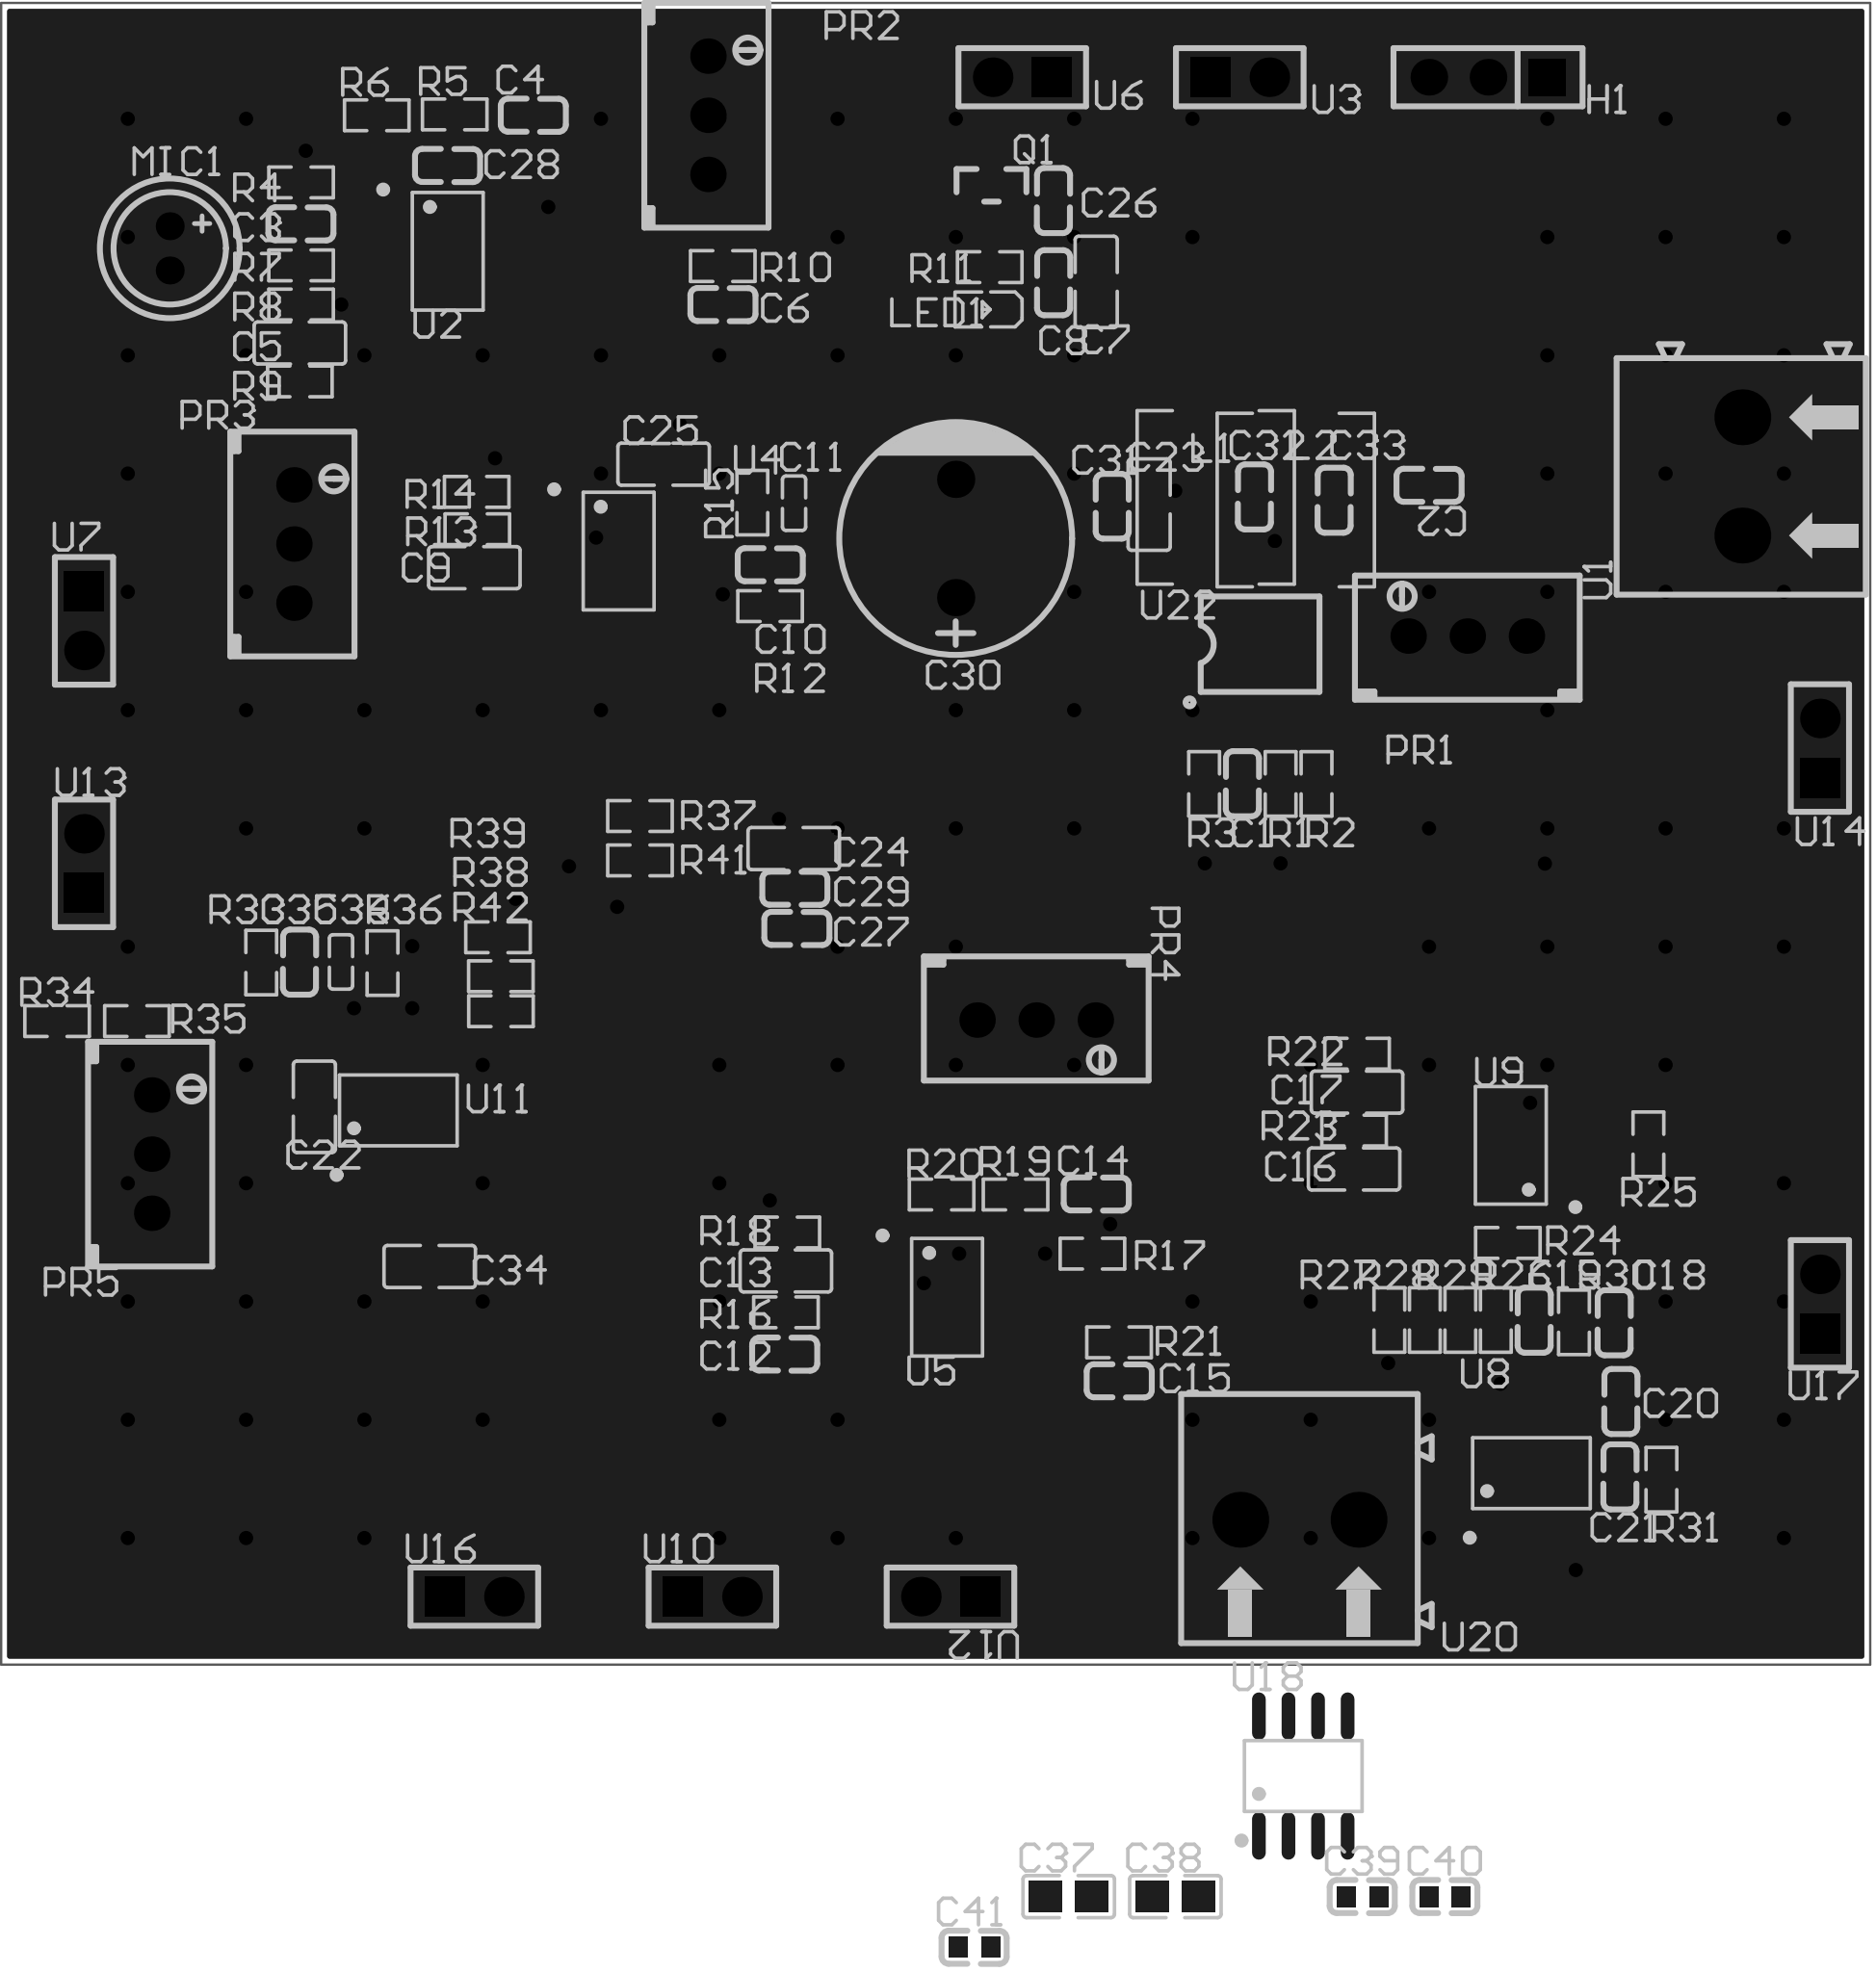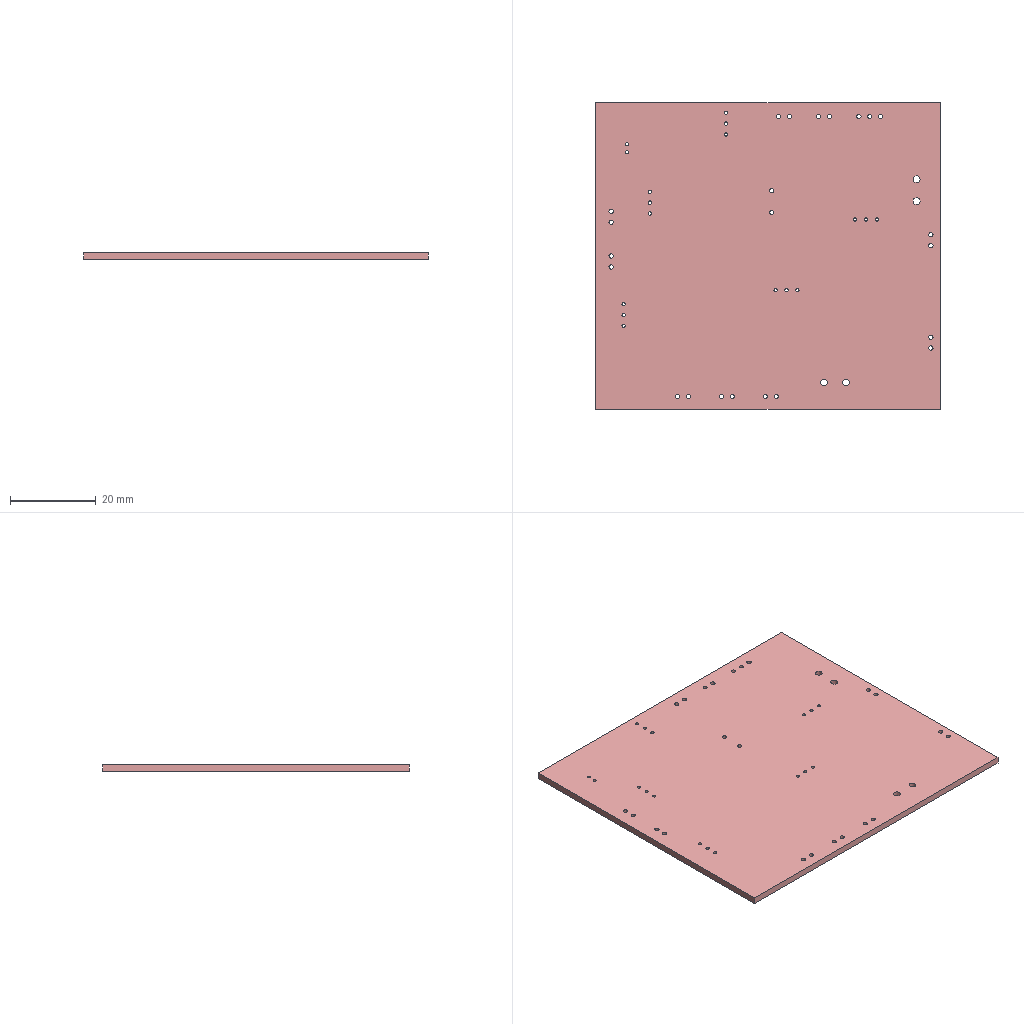Circuit board layout | Altium Designer | box 80.3 x 71.4 x 1.6 mm
Layer stack:
# Altium Designer layer stack of  (unit mm; dielectric type: 0 none, 1 core, 2 prepreg, 3 surface material)
index,name,kind,layer,copper_thickness_mm,dielectric_type,dielectric_thickness_mm,dielectric_material,dielectric_constant
0,Top Paste Mask Layer,other,,,,,,
1,Top Silkscreen Layer,other,,,,,,
2,Top Solder Mask Layer,dielectric,,,3,0.01,,3.3
3,Top Layer,copper,Top Layer,0.035,,,,
4,Dielectric1,dielectric,,,3,1.51,FR4,4.5
5,Bottom Layer,copper,Bottom Layer,0.035,,,,
6,Bottom Solder Mask Layer,dielectric,,,3,0.01,,3.3
7,Bottom Silkscreen Layer,other,,,,,,
8,Bottom Paste Mask Layer,other,,,,,,
# drill layer pairs: low layer,high layer
drill_pair,Top Layer,Bottom Layer
Part placement:
Designator,Comment,Layer,Footprint,Center-X(mm),Center-Y(mm),Rotation
C30,470uF,TopLayer,CAP-TH_BD10.0-P5.00-D1.0-FD,127.987,137.425,90
C31,1uF,TopLayer,C0603,134.709,138.809,90
H1,PM254V-11-03-H85,TopLayer,HDR-TH_3P-P2.54-V-F,150.846,157.237,180
MIC1,GMI6050P-36db,TopLayer,MIC-TH_BD6.0-P1.90-D0.4-L-FD_GMI6050P-2CXXDB,94.234,149.887,270
Q1,AO3401A,TopLayer,SOT-23_L2.9-W1.3-P1.90-LS2.4-BR,129.522,152.595,270
U1,KF128-5.08-2P-AA,TopLayer,CONN-TH_P5.08_KF128-5.08-2P,161.768,140.092,90
U2,NE5532DR,TopLayer,SOIC-8_L4.9-W3.9-P1.27-LS6.0-BL,106.172,149.761,270
U3,ZX-PM2.54-1-2PY,TopLayer,HDR-TH_2P-P2.54-V-F,140.185,157.237,0
U4,NE5532DR,TopLayer,SOIC-8_L4.9-W3.9-P1.27-LS6.0-BL,113.512,136.884,270
U5,NE5532DR,TopLayer,SOIC-8_L4.9-W3.9-P1.27-LS6.0-BL,127.616,104.834,270
U6,ZX-PM2.54-1-2PY,TopLayer,HDR-TH_2P-P2.54-V-F,130.845,157.237,180
U7,ZX-PM2.54-1-2PY,TopLayer,HDR-TH_2P-P2.54-V-F,90.551,133.886,270
U8,NE5532DR,TopLayer,SOIC-8_L4.9-W3.9-P1.27-LS6.0-BL,152.712,97.278,0
U9,NE5532DR,TopLayer,SOIC-8_L4.9-W3.9-P1.27-LS6.0-BL,151.825,111.359,90
U10,ZX-PM2.54-1-2PY,TopLayer,HDR-TH_2P-P2.54-V-F,117.538,91.975,0
U11,NE5532DR,TopLayer,SOIC-8_L4.9-W3.9-P1.27-LS6.0-BL,104.05,112.86,0
U12,ZX-PM2.54-1-2PY,TopLayer,HDR-TH_2P-P2.54-V-F,127.762,91.975,180
U13,ZX-PM2.54-1-2PY,TopLayer,HDR-TH_2P-P2.54-V-F,90.551,123.472,90
U14,ZX-PM2.54-1-2PY,TopLayer,HDR-TH_2P-P2.54-V-F,165.1,128.424,90
U16,ZX-PM2.54-1-2PY,TopLayer,HDR-TH_2P-P2.54-V-F,107.315,91.975,0
U17,ZX-PM2.54-1-2PY,TopLayer,HDR-TH_2P-P2.54-V-F,165.1,104.549,90
U20,KF128-5.08-2P-AA,TopLayer,CONN-TH_P5.08_KF128-5.08-2P,142.748,95.278,0
U22,XPT8871MS,TopLayer,ESOP-8_L4.9-W3.9-P1.27-LS6.0-BL-EP,141.059,132.886,0
C1,1uF,TopLayer,C0603,140.297,126.884,270
C2,470nF,TopLayer,C0603,148.306,139.711,180
C3,1uF,TopLayer,C0603,99.874,150.937,0
C4,1uF,TopLayer,C0603,109.855,155.602,0
C5,100nF,TopLayer,C0805,99.822,145.823,0
C6,1uF,TopLayer,C0603,117.983,147.475,180
C7,100nF,TopLayer,C0805,134.019,148.445,270
C8,1uF,TopLayer,C0603,132.189,148.404,270
C9,100nF,TopLayer,C0805,107.315,136.172,0
C10,1uF,TopLayer,C0603,120.015,136.298,180
C11,3.3pF,TopLayer,C0402,121.044,138.941,90
C12,1uF,TopLayer,C0603,120.65,102.389,0
C13,100nF,TopLayer,C0805,120.692,105.965,180
C14,1uF,TopLayer,C0603,134.03,109.267,0
C15,1uF,TopLayer,C0603,135.001,101.246,180
C16,2.2nF,TopLayer,C0805,145.094,110.343,180
C17,2.2nF,TopLayer,C0805,145.221,113.645,180
C18,27nF,TopLayer,C0603,156.261,103.73,270
C19,27nF,TopLayer,C0603,152.832,103.857,90
C20,68nF,TopLayer,C0603,156.554,100.363,90
C21,68nF,TopLayer,C0603,156.515,97.126,90
C22,100nF,TopLayer,C0805,100.445,113.014,90
C23,100nF,TopLayer,C0805,136.294,138.881,90
C24,100nF,TopLayer,C0805,121.031,124.106,180
C25,100nF,TopLayer,C0805,115.443,140.617,0
C26,10uF,TopLayer,C0603,132.182,151.932,270
C27,10uF,TopLayer,C0603,121.158,120.677,180
C28,10uF,TopLayer,C0603,106.172,153.444,0
C29,10uF,TopLayer,C0603,121.071,122.403,180
C32,1uF,TopLayer,C0603,140.814,139.203,270
C33,1uF,TopLayer,C0603,144.243,139.076,90
C34,100nF,TopLayer,C0805,105.398,106.156,180
C35,1uF,TopLayer,C0603,99.81,119.237,90
C36,3.3pF,TopLayer,C0402,101.588,119.237,270
C37,100nF,TopLayer,C0805,132.841,79.09,0
C38,100nF,TopLayer,C0805,137.42,79.09,0
C39,10uF,TopLayer,C0603,145.452,79.09,0
C40,10uF,TopLayer,C0603,149.001,79.09,0
C41,6.8nF,TopLayer,C0603,128.784,76.91,0
L1,33uH,TopLayer,IND-SMD_L7.3-W6.6,139.154,139.19,90
L2,33uH,TopLayer,IND-SMD_L7.3-W6.6,142.591,139.076,90
LED1,NCD0603G1,TopLayer,LED0603-RD,129.347,147.268,180
PR1,500kΩ,TopLayer,RES-ADJ-TH_3296W,149.958,133.234,90
PR2,10kΩ,TopLayer,RES-ADJ-TH_3296W,117.348,155.602,0
PR3,10kΩ,TopLayer,RES-ADJ-TH_3296W,99.568,137.188,0
PR4,10kΩ,TopLayer,RES-ADJ-TH_3296W,131.445,116.74,270
PR5,10kΩ,TopLayer,RES-ADJ-TH_3296W,93.46,110.982,0
R1,10kΩ,TopLayer,R0603,141.939,126.884,270
R2,10kΩ,TopLayer,R0603,143.481,126.884,90
R3,10kΩ,TopLayer,R0603,138.655,126.884,270
R4,10kΩ,TopLayer,R0603,99.874,152.719,0
R5,0603WAF1001T5E,TopLayer,R0603,106.472,155.64,0
R6,20kΩ,TopLayer,R0603,103.124,155.602,0
R7,0603WAF7502T5E,TopLayer,R0603,99.874,149.156,0
R8,47kΩ,TopLayer,R0603,99.874,147.475,0
R9,47kΩ,TopLayer,R0603,99.822,144.173,180
R10,0603WAF1001T5E,TopLayer,R0603,117.983,149.125,180
R11,10kΩ,TopLayer,R0603,129.447,149.08,180
R12,100kΩ,TopLayer,R0603,120.015,134.52,180
R13,0Ω,TopLayer,R0603,107.442,137.822,0
R14,0603WAF1001T5E,TopLayer,R0603,107.416,139.427,0
R15,1MΩ,TopLayer,R0603,119.253,138.965,90
R16,0603WAF7502T5E,TopLayer,R0603,120.695,104.187,180
R17,47kΩ,TopLayer,R0603,133.858,106.707,180
R18,47kΩ,TopLayer,R0603,120.756,107.616,180
R19,0603WAF1001T5E,TopLayer,R0603,130.556,109.248,0
R20,20kΩ,TopLayer,R0603,127.381,109.248,180
R21,0603WAF1001T5E,TopLayer,R0603,135.001,102.897,0
R22,20kΩ,TopLayer,R0603,145.221,115.296,0
R23,20kΩ,TopLayer,R0603,145.094,111.994,180
R24,20kΩ,TopLayer,R0603,151.698,107.168,180
R25,20kΩ,TopLayer,R0603,157.734,111.406,90
R26,20kΩ,TopLayer,R0603,151.181,103.857,90
R27,0603WAF1001T5E,TopLayer,R0603,146.609,103.857,270
R28,11kΩ,TopLayer,R0603,148.133,103.857,90
R29,20kΩ,TopLayer,R0603,149.657,103.857,270
R30,16kΩ,TopLayer,R0603,154.537,103.757,90
R31,0603WAF3001T5E,TopLayer,R0603,158.293,96.999,90
R33,100kΩ,TopLayer,R0603,98.163,119.21,90
R34,0Ω,TopLayer,R0603,89.396,116.697,180
R35,0603WAF1001T5E,TopLayer,R0603,92.825,116.697,0
R36,1MΩ,TopLayer,R0603,103.37,119.188,270
R37,10kΩ,TopLayer,R0603,114.427,125.504,0
R38,10kΩ,TopLayer,R0603,108.453,118.621,0
R39,10kΩ,TopLayer,R0603,108.331,120.296,0
R41,10kΩ,TopLayer,R0603,114.427,123.599,0
R42,10kΩ,TopLayer,R0603,108.458,117.121,0
U18,NE5532DR,TopLayer,SOIC-8_L4.9-W3.9-P1.27-LS6.0-BL,142.912,84.269,0
Pad and via stacks:
# Altium Designer via and pad stacks of  (unit mm). Each distinct definition once, with the count of objects using it.
# via: kind,start_layer,end_layer,hole_mm,diameter_mm,mode(0 simple;1 top-mid-bottom;2 full stack),diameter_per_layer,count,example_net
# pad: kind,layer,hole_mm,hole_type(0 round;1 square;2 slot),plating,top_size,top_shape(1 round;2 rect;3 octagon;9 rounded rect),mid_size,bottom_size,mode,footprint,size_per_layer,count,example
pad,Multi-Layer,1,0,plated,1.6x1.6,1,1.6x1.6,1.6x1.6,0,CAP-TH_BD10.0-P5.00-D1.0-FD,,2,C30.1
pad,Multi-Layer,1.02,0,plated,1.575x1.575,1,1.575x1.575,1.575x1.575,0,HDR-TH_3P-P2.54-V-F,,2,H1.3
pad,Multi-Layer,1.02,0,plated,1.575x1.575,2,1.575x1.575,1.575x1.575,0,HDR-TH_3P-P2.54-V-F,,1,H1.1
pad,Multi-Layer,0.7,0,plated,1.2x1.2,1,1.2x1.2,1.2x1.2,0,MIC-TH_BD6.0-P1.90-D0.4-L-FD_GMI6050P-2CXXDB,,2,MIC1.1
pad,Multi-Layer,1.6,0,plated,2.4x2.4,1,2.4x2.4,2.4x2.4,0,CONN-TH_P5.08_KF128-5.08-2P,,4,U1.1
pad,Multi-Layer,1,0,plated,1.7x1.7,2,1.7x1.7,1.7x1.7,0,HDR-TH_2P-P2.54-V-F,,9,U3.1
pad,Multi-Layer,1,0,plated,1.7x1.7,1,1.7x1.7,1.7x1.7,0,HDR-TH_2P-P2.54-V-F,,9,U3.2
pad,Multi-Layer,0.762,0,plated,1.524x1.524,1,1.524x1.524,1.524x1.524,0,RES-ADJ-TH_3296W,,15,PR1.2
pad,Top Layer,0,0,plated,0.8x0.9,2,0.8x0.9,0.8x0.9,0,C0603,,50,C31.2
pad,Top Layer,0,0,plated,1x0.8,2,1x0.8,1x0.8,0,SOT-23_L2.9-W1.3-P1.90-LS2.4-BR,,3,Q1.2
pad,Top Layer,0,0,plated,0.588x2.045,1,0.588x2.045,0.588x2.045,0,SOIC-8_L4.9-W3.9-P1.27-LS6.0-BL,,56,U2.5
pad,Top Layer,0,0,plated,0.6x1.2,2,0.6x1.2,0.6x1.2,0,ESOP-8_L4.9-W3.9-P1.27-LS6.0-BL-EP,,8,U22.1
pad,Top Layer,0,0,plated,3.3x2.4,2,3.3x2.4,3.3x2.4,0,ESOP-8_L4.9-W3.9-P1.27-LS6.0-BL-EP,,1,U22.9
pad,Top Layer,0,0,plated,1.41x1.35,2,1.41x1.35,1.41x1.35,0,C0805,,26,C5.2
pad,Top Layer,0,0,plated,0.7901x0.54,2,0.7901x0.54,0.7901x0.54,0,C0402,,4,C11.2
pad,Top Layer,0,0,plated,2.423x3.419,2,2.423x3.419,2.423x3.419,0,IND-SMD_L7.3-W6.6,,4,L1.1
pad,Top Layer,0,0,plated,0.8x0.8,2,0.8x0.8,0.8x0.8,0,LED0603-RD,,2,LED1.2
pad,Top Layer,0,0,plated,0.8065x0.864,2,0.8065x0.864,0.8065x0.864,0,R0603,,80,R1.2
via,Top Layer,Bottom Layer,0.3048,0.61,0,,148,$1N133
Copper pours:
name,layer,net,type(0 solid;1 hatched;2 none)
Top Layer-GND,Top Layer,GND,0
Bottom Layer-GND,Bottom Layer,GND,0
Design rules, without the lines most boards share:
# Altium Designer design rules of  (exported by Altium Designer, unit mm)
# columns: name | kind | enabled | priority | scope1 | scope2 | descriptor | typed fields (field=value)
creepage | 65 | enabled | 1 | All | All | Creepage Distance Constraint =(0mil) (All),(All) |
copperRegion | 20 | enabled | 1 | (InNet('GND')) | All | Polygon Connect Rule(Relief Connect )(Conductor Width=10mil) (Relief Angle=90 Angle) (Entries=4) (Air Gap Width=10mil) ((InNet('GND'))),(All) | connect_style(0=relief,1=direct,2=none)=0 relief_conductor_width=0.254 relief_entries=4